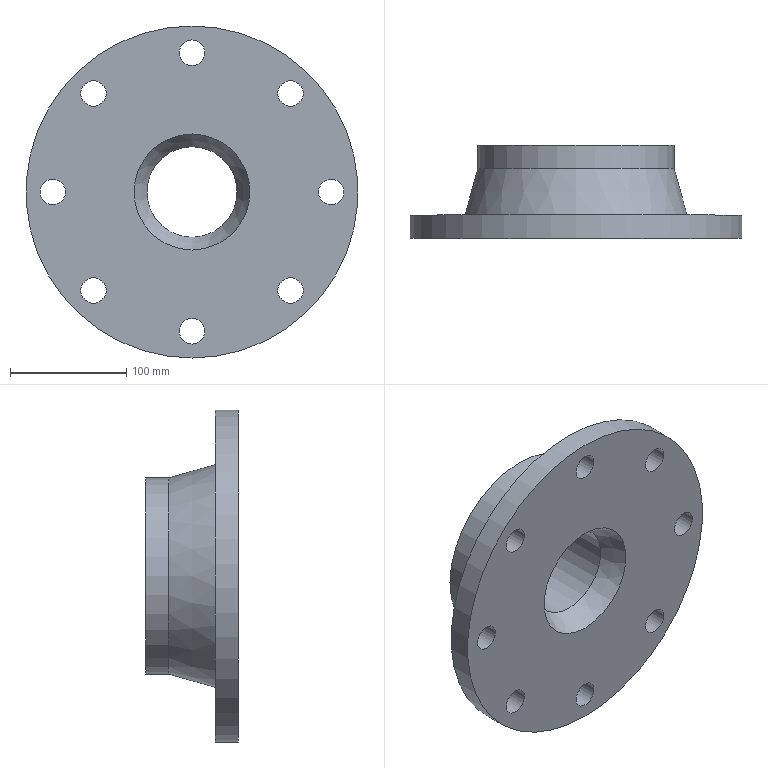Part | NX | features DATUM_CSYS 11, SKETCH 11, EXTRACT_DATUM_AXIS 8, EXTRACT_FACE 8, HOLE PACKAGE 8, SIMPLE HOLE 8, Instance Feature 7, ABSOLUTE_DATUM_PLANE 3, Resize Face 3, CPROJ 2, SWP104 2, ABSOLUTE_DATUM_AXIS 1, BLEND 1, EXTRUDE 1, Pattern Feature 1 | 2 solids | 24 faces | box 286 x 80 x 286 mm | volume 2285168 mm3 | cylinder 11 | plane 6 | cone 4 | torus 3 | commonest cylinder face diameters 22 x8 78 x1 169 x1 286 x1
STEP:
#1=CARTESIAN_POINT('',(0.,46.129,-75.847));
#2=VERTEX_POINT('',#1);
#3=CARTESIAN_POINT('',(0.,46.129,0.));
#4=DIRECTION('',(0.,-1.,0.));
#5=DIRECTION('',(0.,0.,-1.));
#6=AXIS2_PLACEMENT_3D('',#3,#4,#5);
#7=CIRCLE('',#6,75.847);
#8=EDGE_CURVE('',#2,#2,#7,.T.);
#9=ORIENTED_EDGE('',*,*,#8,.T.);
#10=EDGE_LOOP('',(#9));
#11=FACE_BOUND('',#10,.T.);
#12=CARTESIAN_POINT('',(0.,83.956,-65.03));
#13=VERTEX_POINT('',#12);
#14=CARTESIAN_POINT('',(0.,83.956,0.));
#15=DIRECTION('',(0.,-1.,0.));
#16=DIRECTION('',(0.,0.,-1.));
#17=AXIS2_PLACEMENT_3D('',#14,#15,#16);
#18=CIRCLE('',#17,65.03);
#19=EDGE_CURVE('',#13,#13,#18,.T.);
#20=ORIENTED_EDGE('',*,*,#19,.F.);
#21=EDGE_LOOP('',(#20));
#22=FACE_BOUND('',#21,.T.);
#23=CARTESIAN_POINT('',(0.,83.956,0.));
#24=DIRECTION('',(0.,-1.,0.));
#25=DIRECTION('',(0.,0.,-1.));
#26=AXIS2_PLACEMENT_3D('',#23,#24,#25);
#27=CONICAL_SURFACE('',#26,65.03,0.2785);
#28=ADVANCED_FACE('',(#11,#22),#27,.F.);
#29=CARTESIAN_POINT('',(0.,43.956,-78.73));
#30=VERTEX_POINT('',#29);
#31=CARTESIAN_POINT('',(0.,43.956,0.));
#32=DIRECTION('',(0.,-1.,0.));
#33=DIRECTION('',(0.,0.,-1.));
#34=AXIS2_PLACEMENT_3D('',#31,#32,#33);
#35=CIRCLE('',#34,78.73);
#36=EDGE_CURVE('',#30,#30,#35,.T.);
#37=ORIENTED_EDGE('',*,*,#36,.T.);
#38=EDGE_LOOP('',(#37));
#39=FACE_BOUND('',#38,.T.);
#40=ORIENTED_EDGE('',*,*,#8,.F.);
#41=EDGE_LOOP('',(#40));
#42=FACE_BOUND('',#41,.T.);
#43=CARTESIAN_POINT('',(0.,46.956,0.));
#44=DIRECTION('',(0.,-1.,0.));
#45=DIRECTION('',(0.,0.,-1.));
#46=AXIS2_PLACEMENT_3D('',#43,#44,#45);
#47=TOROIDAL_SURFACE('',#46,78.73,3.);
#48=ADVANCED_FACE('',(#39,#42),#47,.T.);
#49=CARTESIAN_POINT('',(0.,43.956,-95.938));
#50=VERTEX_POINT('',#49);
#51=CARTESIAN_POINT('',(0.,43.956,0.));
#52=DIRECTION('',(0.,-1.,0.));
#53=DIRECTION('',(0.,0.,-1.));
#54=AXIS2_PLACEMENT_3D('',#51,#52,#53);
#55=CIRCLE('',#54,95.938);
#56=EDGE_CURVE('',#50,#50,#55,.T.);
#57=ORIENTED_EDGE('',*,*,#56,.T.);
#58=EDGE_LOOP('',(#57));
#59=FACE_BOUND('',#58,.T.);
#60=ORIENTED_EDGE('',*,*,#36,.F.);
#61=EDGE_LOOP('',(#60));
#62=FACE_BOUND('',#61,.T.);
#63=CARTESIAN_POINT('',(78.73,43.956,0.));
#64=DIRECTION('',(0.,-1.,0.));
#65=DIRECTION('',(0.,0.,-1.));
#66=AXIS2_PLACEMENT_3D('',#63,#64,#65);
#67=PLANE('',#66);
#68=ADVANCED_FACE('',(#59,#62),#67,.T.);
#69=CARTESIAN_POINT('',(0.,83.956,-84.5));
#70=VERTEX_POINT('',#69);
#71=CARTESIAN_POINT('',(0.,83.956,0.));
#72=DIRECTION('',(0.,-1.,0.));
#73=DIRECTION('',(0.,0.,-1.));
#74=AXIS2_PLACEMENT_3D('',#71,#72,#73);
#75=CIRCLE('',#74,84.5);
#76=EDGE_CURVE('',#70,#70,#75,.T.);
#77=ORIENTED_EDGE('',*,*,#76,.T.);
#78=EDGE_LOOP('',(#77));
#79=FACE_BOUND('',#78,.T.);
#80=ORIENTED_EDGE('',*,*,#56,.F.);
#81=EDGE_LOOP('',(#80));
#82=FACE_BOUND('',#81,.T.);
#83=CARTESIAN_POINT('',(0.,43.956,0.));
#84=DIRECTION('',(0.,-1.,0.));
#85=DIRECTION('',(0.,0.,-1.));
#86=AXIS2_PLACEMENT_3D('',#83,#84,#85);
#87=CONICAL_SURFACE('',#86,95.938,0.2785);
#88=ADVANCED_FACE('',(#79,#82),#87,.T.);
#89=ORIENTED_EDGE('',*,*,#19,.T.);
#90=EDGE_LOOP('',(#89));
#91=FACE_BOUND('',#90,.T.);
#92=ORIENTED_EDGE('',*,*,#76,.F.);
#93=EDGE_LOOP('',(#92));
#94=FACE_BOUND('',#93,.T.);
#95=CARTESIAN_POINT('',(84.5,83.956,0.));
#96=DIRECTION('',(0.,1.,0.));
#97=DIRECTION('',(0.,0.,1.));
#98=AXIS2_PLACEMENT_3D('',#95,#96,#97);
#99=PLANE('',#98);
#100=ADVANCED_FACE('',(#91,#94),#99,.T.);
#101=CLOSED_SHELL('',(#28,#48,#68,#88,#100));
#102=MANIFOLD_SOLID_BREP('',#101);
#103=CARTESIAN_POINT('',(0.,83.55,-65.116));
#104=VERTEX_POINT('',#103);
#105=CARTESIAN_POINT('',(0.,83.55,0.));
#106=DIRECTION('',(0.,-1.,0.));
#107=DIRECTION('',(0.,0.,-1.));
#108=AXIS2_PLACEMENT_3D('',#105,#106,#107);
#109=CIRCLE('',#108,65.116);
#110=EDGE_CURVE('',#104,#104,#109,.T.);
#111=ORIENTED_EDGE('',*,*,#110,.F.);
#112=EDGE_LOOP('',(#111));
#113=FACE_BOUND('',#112,.T.);
#114=CARTESIAN_POINT('',(0.,83.956,-65.03));
#115=VERTEX_POINT('',#114);
#116=CARTESIAN_POINT('',(0.,83.956,0.));
#117=DIRECTION('',(0.,-1.,0.));
#118=DIRECTION('',(0.,0.,-1.));
#119=AXIS2_PLACEMENT_3D('',#116,#117,#118);
#120=CIRCLE('',#119,65.03);
#121=EDGE_CURVE('',#115,#115,#120,.F.);
#122=ORIENTED_EDGE('',*,*,#121,.F.);
#123=EDGE_LOOP('',(#122));
#124=FACE_BOUND('',#123,.T.);
#125=CARTESIAN_POINT('',(0.,84.377,0.));
#126=DIRECTION('',(0.,1.,0.));
#127=DIRECTION('',(0.,0.,1.));
#128=AXIS2_PLACEMENT_3D('',#125,#126,#127);
#129=TOROIDAL_SURFACE('',#128,68.,3.);
#130=ADVANCED_FACE('',(#113,#124),#129,.F.);
#131=CARTESIAN_POINT('',(-84.853,23.956,-73.853));
#132=VERTEX_POINT('',#131);
#133=CARTESIAN_POINT('',(-84.853,23.956,-84.853));
#134=DIRECTION('',(0.,1.,0.));
#135=DIRECTION('',(0.,0.,1.));
#136=AXIS2_PLACEMENT_3D('',#133,#134,#135);
#137=CIRCLE('',#136,11.);
#138=EDGE_CURVE('',#132,#132,#137,.T.);
#139=ORIENTED_EDGE('',*,*,#138,.T.);
#140=EDGE_LOOP('',(#139));
#141=FACE_BOUND('',#140,.T.);
#142=CARTESIAN_POINT('',(0.,23.956,-109.));
#143=VERTEX_POINT('',#142);
#144=CARTESIAN_POINT('',(0.,23.956,-120.));
#145=DIRECTION('',(0.,1.,0.));
#146=DIRECTION('',(0.,0.,1.));
#147=AXIS2_PLACEMENT_3D('',#144,#145,#146);
#148=CIRCLE('',#147,11.);
#149=EDGE_CURVE('',#143,#143,#148,.T.);
#150=ORIENTED_EDGE('',*,*,#149,.T.);
#151=EDGE_LOOP('',(#150));
#152=FACE_BOUND('',#151,.T.);
#153=CARTESIAN_POINT('',(84.853,23.956,-73.853));
#154=VERTEX_POINT('',#153);
#155=CARTESIAN_POINT('',(84.853,23.956,-84.853));
#156=DIRECTION('',(0.,1.,0.));
#157=DIRECTION('',(0.,0.,1.));
#158=AXIS2_PLACEMENT_3D('',#155,#156,#157);
#159=CIRCLE('',#158,11.);
#160=EDGE_CURVE('',#154,#154,#159,.T.);
#161=ORIENTED_EDGE('',*,*,#160,.T.);
#162=EDGE_LOOP('',(#161));
#163=FACE_BOUND('',#162,.T.);
#164=CARTESIAN_POINT('',(120.,23.956,11.));
#165=VERTEX_POINT('',#164);
#166=CARTESIAN_POINT('',(120.,23.956,0.));
#167=DIRECTION('',(0.,1.,0.));
#168=DIRECTION('',(0.,0.,1.));
#169=AXIS2_PLACEMENT_3D('',#166,#167,#168);
#170=CIRCLE('',#169,11.);
#171=EDGE_CURVE('',#165,#165,#170,.T.);
#172=ORIENTED_EDGE('',*,*,#171,.T.);
#173=EDGE_LOOP('',(#172));
#174=FACE_BOUND('',#173,.T.);
#175=CARTESIAN_POINT('',(84.853,23.956,95.853));
#176=VERTEX_POINT('',#175);
#177=CARTESIAN_POINT('',(84.853,23.956,84.853));
#178=DIRECTION('',(0.,1.,0.));
#179=DIRECTION('',(0.,0.,1.));
#180=AXIS2_PLACEMENT_3D('',#177,#178,#179);
#181=CIRCLE('',#180,11.);
#182=EDGE_CURVE('',#176,#176,#181,.T.);
#183=ORIENTED_EDGE('',*,*,#182,.T.);
#184=EDGE_LOOP('',(#183));
#185=FACE_BOUND('',#184,.T.);
#186=CARTESIAN_POINT('',(0.,23.956,131.));
#187=VERTEX_POINT('',#186);
#188=CARTESIAN_POINT('',(0.,23.956,120.));
#189=DIRECTION('',(0.,1.,0.));
#190=DIRECTION('',(0.,0.,1.));
#191=AXIS2_PLACEMENT_3D('',#188,#189,#190);
#192=CIRCLE('',#191,11.);
#193=EDGE_CURVE('',#187,#187,#192,.T.);
#194=ORIENTED_EDGE('',*,*,#193,.T.);
#195=EDGE_LOOP('',(#194));
#196=FACE_BOUND('',#195,.T.);
#197=CARTESIAN_POINT('',(-84.853,23.956,95.853));
#198=VERTEX_POINT('',#197);
#199=CARTESIAN_POINT('',(-84.853,23.956,84.853));
#200=DIRECTION('',(0.,1.,0.));
#201=DIRECTION('',(0.,0.,1.));
#202=AXIS2_PLACEMENT_3D('',#199,#200,#201);
#203=CIRCLE('',#202,11.);
#204=EDGE_CURVE('',#198,#198,#203,.T.);
#205=ORIENTED_EDGE('',*,*,#204,.T.);
#206=EDGE_LOOP('',(#205));
#207=FACE_BOUND('',#206,.T.);
#208=CARTESIAN_POINT('',(-120.,23.956,11.));
#209=VERTEX_POINT('',#208);
#210=CARTESIAN_POINT('',(-120.,23.956,0.));
#211=DIRECTION('',(0.,1.,0.));
#212=DIRECTION('',(0.,0.,1.));
#213=AXIS2_PLACEMENT_3D('',#210,#211,#212);
#214=CIRCLE('',#213,11.);
#215=EDGE_CURVE('',#209,#209,#214,.T.);
#216=ORIENTED_EDGE('',*,*,#215,.T.);
#217=EDGE_LOOP('',(#216));
#218=FACE_BOUND('',#217,.T.);
#219=CARTESIAN_POINT('',(0.,23.956,-50.));
#220=VERTEX_POINT('',#219);
#221=CARTESIAN_POINT('',(0.,23.956,0.));
#222=DIRECTION('',(0.,-1.,0.));
#223=DIRECTION('',(0.,0.,-1.));
#224=AXIS2_PLACEMENT_3D('',#221,#222,#223);
#225=CIRCLE('',#224,50.);
#226=EDGE_CURVE('',#220,#220,#225,.T.);
#227=ORIENTED_EDGE('',*,*,#226,.F.);
#228=EDGE_LOOP('',(#227));
#229=FACE_BOUND('',#228,.T.);
#230=CARTESIAN_POINT('',(0.,23.956,143.));
#231=VERTEX_POINT('',#230);
#232=CARTESIAN_POINT('',(0.,23.956,0.));
#233=DIRECTION('',(0.,1.,0.));
#234=DIRECTION('',(0.,0.,1.));
#235=AXIS2_PLACEMENT_3D('',#232,#233,#234);
#236=CIRCLE('',#235,143.);
#237=EDGE_CURVE('',#231,#231,#236,.F.);
#238=ORIENTED_EDGE('',*,*,#237,.T.);
#239=EDGE_LOOP('',(#238));
#240=FACE_BOUND('',#239,.T.);
#241=CARTESIAN_POINT('',(110.,23.956,0.));
#242=DIRECTION('',(0.,1.,0.));
#243=DIRECTION('',(0.,0.,1.));
#244=AXIS2_PLACEMENT_3D('',#241,#242,#243);
#245=PLANE('',#244);
#246=ADVANCED_FACE('',(#141,#152,#163,#174,#185,#196,#207,#218,#229,#240),#245,.F.);
#247=CARTESIAN_POINT('',(0.,43.756,-39.));
#248=VERTEX_POINT('',#247);
#249=CARTESIAN_POINT('',(0.,43.756,0.));
#250=DIRECTION('',(0.,-1.,0.));
#251=DIRECTION('',(0.,0.,-1.));
#252=AXIS2_PLACEMENT_3D('',#249,#250,#251);
#253=CIRCLE('',#252,39.);
#254=EDGE_CURVE('',#248,#248,#253,.T.);
#255=ORIENTED_EDGE('',*,*,#254,.F.);
#256=EDGE_LOOP('',(#255));
#257=FACE_BOUND('',#256,.T.);
#258=ORIENTED_EDGE('',*,*,#226,.T.);
#259=EDGE_LOOP('',(#258));
#260=FACE_BOUND('',#259,.T.);
#261=CARTESIAN_POINT('',(0.,23.956,0.));
#262=DIRECTION('',(0.,-1.,0.));
#263=DIRECTION('',(0.,0.,-1.));
#264=AXIS2_PLACEMENT_3D('',#261,#262,#263);
#265=CONICAL_SURFACE('',#264,50.,0.5071);
#266=ADVANCED_FACE('',(#257,#260),#265,.F.);
#267=CARTESIAN_POINT('',(0.,103.956,-39.));
#268=VERTEX_POINT('',#267);
#269=CARTESIAN_POINT('',(0.,103.956,0.));
#270=DIRECTION('',(0.,-1.,0.));
#271=DIRECTION('',(0.,0.,-1.));
#272=AXIS2_PLACEMENT_3D('',#269,#270,#271);
#273=CIRCLE('',#272,39.);
#274=EDGE_CURVE('',#268,#268,#273,.T.);
#275=ORIENTED_EDGE('',*,*,#274,.F.);
#276=EDGE_LOOP('',(#275));
#277=FACE_BOUND('',#276,.T.);
#278=ORIENTED_EDGE('',*,*,#254,.T.);
#279=EDGE_LOOP('',(#278));
#280=FACE_BOUND('',#279,.T.);
#281=CARTESIAN_POINT('',(0.,0.,0.));
#282=DIRECTION('',(0.,-1.,0.));
#283=DIRECTION('',(0.,0.,-1.));
#284=AXIS2_PLACEMENT_3D('',#281,#282,#283);
#285=CYLINDRICAL_SURFACE('',#284,39.);
#286=ADVANCED_FACE('',(#277,#280),#285,.F.);
#287=ORIENTED_EDGE('',*,*,#274,.T.);
#288=EDGE_LOOP('',(#287));
#289=FACE_BOUND('',#288,.T.);
#290=CARTESIAN_POINT('',(0.,103.956,84.5));
#291=VERTEX_POINT('',#290);
#292=CARTESIAN_POINT('',(0.,103.956,0.));
#293=DIRECTION('',(0.,1.,0.));
#294=DIRECTION('',(0.,0.,1.));
#295=AXIS2_PLACEMENT_3D('',#292,#293,#294);
#296=CIRCLE('',#295,84.5);
#297=EDGE_CURVE('',#291,#291,#296,.T.);
#298=ORIENTED_EDGE('',*,*,#297,.T.);
#299=EDGE_LOOP('',(#298));
#300=FACE_BOUND('',#299,.T.);
#301=CARTESIAN_POINT('',(20.,103.956,0.));
#302=DIRECTION('',(0.,-1.,0.));
#303=DIRECTION('',(0.,0.,-1.));
#304=AXIS2_PLACEMENT_3D('',#301,#302,#303);
#305=PLANE('',#304);
#306=ADVANCED_FACE('',(#289,#300),#305,.F.);
#307=CARTESIAN_POINT('',(0.,46.129,-75.847));
#308=VERTEX_POINT('',#307);
#309=CARTESIAN_POINT('',(0.,46.129,0.));
#310=DIRECTION('',(0.,-1.,0.));
#311=DIRECTION('',(0.,0.,-1.));
#312=AXIS2_PLACEMENT_3D('',#309,#310,#311);
#313=CIRCLE('',#312,75.847);
#314=EDGE_CURVE('',#308,#308,#313,.F.);
#315=ORIENTED_EDGE('',*,*,#314,.T.);
#316=EDGE_LOOP('',(#315));
#317=FACE_BOUND('',#316,.T.);
#318=ORIENTED_EDGE('',*,*,#110,.T.);
#319=EDGE_LOOP('',(#318));
#320=FACE_BOUND('',#319,.T.);
#321=CARTESIAN_POINT('',(0.,83.956,0.));
#322=DIRECTION('',(0.,-1.,0.));
#323=DIRECTION('',(0.,0.,-1.));
#324=AXIS2_PLACEMENT_3D('',#321,#322,#323);
#325=CONICAL_SURFACE('',#324,65.,0.2793);
#326=ADVANCED_FACE('',(#317,#320),#325,.T.);
#327=CARTESIAN_POINT('',(-84.853,43.956,-95.853));
#328=VERTEX_POINT('',#327);
#329=CARTESIAN_POINT('',(-84.853,43.956,-84.853));
#330=DIRECTION('',(0.,-1.,0.));
#331=DIRECTION('',(0.,0.,-1.));
#332=AXIS2_PLACEMENT_3D('',#329,#330,#331);
#333=CIRCLE('',#332,11.);
#334=EDGE_CURVE('',#328,#328,#333,.T.);
#335=ORIENTED_EDGE('',*,*,#334,.T.);
#336=EDGE_LOOP('',(#335));
#337=FACE_BOUND('',#336,.T.);
#338=CARTESIAN_POINT('',(0.,43.956,-131.));
#339=VERTEX_POINT('',#338);
#340=CARTESIAN_POINT('',(0.,43.956,-120.));
#341=DIRECTION('',(0.,-1.,0.));
#342=DIRECTION('',(0.,0.,-1.));
#343=AXIS2_PLACEMENT_3D('',#340,#341,#342);
#344=CIRCLE('',#343,11.);
#345=EDGE_CURVE('',#339,#339,#344,.T.);
#346=ORIENTED_EDGE('',*,*,#345,.T.);
#347=EDGE_LOOP('',(#346));
#348=FACE_BOUND('',#347,.T.);
#349=CARTESIAN_POINT('',(84.853,43.956,-95.853));
#350=VERTEX_POINT('',#349);
#351=CARTESIAN_POINT('',(84.853,43.956,-84.853));
#352=DIRECTION('',(0.,-1.,0.));
#353=DIRECTION('',(0.,0.,-1.));
#354=AXIS2_PLACEMENT_3D('',#351,#352,#353);
#355=CIRCLE('',#354,11.);
#356=EDGE_CURVE('',#350,#350,#355,.T.);
#357=ORIENTED_EDGE('',*,*,#356,.T.);
#358=EDGE_LOOP('',(#357));
#359=FACE_BOUND('',#358,.T.);
#360=CARTESIAN_POINT('',(120.,43.956,-11.));
#361=VERTEX_POINT('',#360);
#362=CARTESIAN_POINT('',(120.,43.956,0.));
#363=DIRECTION('',(0.,-1.,0.));
#364=DIRECTION('',(0.,0.,-1.));
#365=AXIS2_PLACEMENT_3D('',#362,#363,#364);
#366=CIRCLE('',#365,11.);
#367=EDGE_CURVE('',#361,#361,#366,.T.);
#368=ORIENTED_EDGE('',*,*,#367,.T.);
#369=EDGE_LOOP('',(#368));
#370=FACE_BOUND('',#369,.T.);
#371=CARTESIAN_POINT('',(84.853,43.956,73.853));
#372=VERTEX_POINT('',#371);
#373=CARTESIAN_POINT('',(84.853,43.956,84.853));
#374=DIRECTION('',(0.,-1.,0.));
#375=DIRECTION('',(0.,0.,-1.));
#376=AXIS2_PLACEMENT_3D('',#373,#374,#375);
#377=CIRCLE('',#376,11.);
#378=EDGE_CURVE('',#372,#372,#377,.T.);
#379=ORIENTED_EDGE('',*,*,#378,.T.);
#380=EDGE_LOOP('',(#379));
#381=FACE_BOUND('',#380,.T.);
#382=CARTESIAN_POINT('',(0.,43.956,109.));
#383=VERTEX_POINT('',#382);
#384=CARTESIAN_POINT('',(0.,43.956,120.));
#385=DIRECTION('',(0.,-1.,0.));
#386=DIRECTION('',(0.,0.,-1.));
#387=AXIS2_PLACEMENT_3D('',#384,#385,#386);
#388=CIRCLE('',#387,11.);
#389=EDGE_CURVE('',#383,#383,#388,.T.);
#390=ORIENTED_EDGE('',*,*,#389,.T.);
#391=EDGE_LOOP('',(#390));
#392=FACE_BOUND('',#391,.T.);
#393=CARTESIAN_POINT('',(-84.853,43.956,73.853));
#394=VERTEX_POINT('',#393);
#395=CARTESIAN_POINT('',(-84.853,43.956,84.853));
#396=DIRECTION('',(0.,-1.,0.));
#397=DIRECTION('',(0.,0.,-1.));
#398=AXIS2_PLACEMENT_3D('',#395,#396,#397);
#399=CIRCLE('',#398,11.);
#400=EDGE_CURVE('',#394,#394,#399,.T.);
#401=ORIENTED_EDGE('',*,*,#400,.T.);
#402=EDGE_LOOP('',(#401));
#403=FACE_BOUND('',#402,.T.);
#404=CARTESIAN_POINT('',(-120.,43.956,-11.));
#405=VERTEX_POINT('',#404);
#406=CARTESIAN_POINT('',(-120.,43.956,0.));
#407=DIRECTION('',(0.,-1.,0.));
#408=DIRECTION('',(0.,0.,-1.));
#409=AXIS2_PLACEMENT_3D('',#406,#407,#408);
#410=CIRCLE('',#409,11.);
#411=EDGE_CURVE('',#405,#405,#410,.T.);
#412=ORIENTED_EDGE('',*,*,#411,.T.);
#413=EDGE_LOOP('',(#412));
#414=FACE_BOUND('',#413,.T.);
#415=CARTESIAN_POINT('',(0.,43.956,-78.73));
#416=VERTEX_POINT('',#415);
#417=CARTESIAN_POINT('',(0.,43.956,0.));
#418=DIRECTION('',(0.,-1.,0.));
#419=DIRECTION('',(0.,0.,-1.));
#420=AXIS2_PLACEMENT_3D('',#417,#418,#419);
#421=CIRCLE('',#420,78.73);
#422=EDGE_CURVE('',#416,#416,#421,.T.);
#423=ORIENTED_EDGE('',*,*,#422,.T.);
#424=EDGE_LOOP('',(#423));
#425=FACE_BOUND('',#424,.T.);
#426=CARTESIAN_POINT('',(0.,43.956,-143.));
#427=VERTEX_POINT('',#426);
#428=CARTESIAN_POINT('',(0.,43.956,0.));
#429=DIRECTION('',(0.,-1.,0.));
#430=DIRECTION('',(0.,0.,-1.));
#431=AXIS2_PLACEMENT_3D('',#428,#429,#430);
#432=CIRCLE('',#431,143.);
#433=EDGE_CURVE('',#427,#427,#432,.T.);
#434=ORIENTED_EDGE('',*,*,#433,.F.);
#435=EDGE_LOOP('',(#434));
#436=FACE_BOUND('',#435,.T.);
#437=CARTESIAN_POINT('',(75.,43.956,0.));
#438=DIRECTION('',(0.,-1.,0.));
#439=DIRECTION('',(0.,0.,-1.));
#440=AXIS2_PLACEMENT_3D('',#437,#438,#439);
#441=PLANE('',#440);
#442=ADVANCED_FACE('',(#337,#348,#359,#370,#381,#392,#403,#414,#425,#436),#441,.F.);
#443=ORIENTED_EDGE('',*,*,#237,.F.);
#444=EDGE_LOOP('',(#443));
#445=FACE_BOUND('',#444,.T.);
#446=ORIENTED_EDGE('',*,*,#433,.T.);
#447=EDGE_LOOP('',(#446));
#448=FACE_BOUND('',#447,.T.);
#449=CARTESIAN_POINT('',(0.,0.,0.));
#450=DIRECTION('',(0.,-1.,0.));
#451=DIRECTION('',(0.,0.,-1.));
#452=AXIS2_PLACEMENT_3D('',#449,#450,#451);
#453=CYLINDRICAL_SURFACE('',#452,143.);
#454=ADVANCED_FACE('',(#445,#448),#453,.T.);
#455=ORIENTED_EDGE('',*,*,#314,.F.);
#456=EDGE_LOOP('',(#455));
#457=FACE_BOUND('',#456,.T.);
#458=ORIENTED_EDGE('',*,*,#422,.F.);
#459=EDGE_LOOP('',(#458));
#460=FACE_BOUND('',#459,.T.);
#461=CARTESIAN_POINT('',(0.,46.956,0.));
#462=DIRECTION('',(0.,-1.,0.));
#463=DIRECTION('',(0.,0.,-1.));
#464=AXIS2_PLACEMENT_3D('',#461,#462,#463);
#465=TOROIDAL_SURFACE('',#464,78.73,3.);
#466=ADVANCED_FACE('',(#457,#460),#465,.F.);
#467=ORIENTED_EDGE('',*,*,#411,.F.);
#468=EDGE_LOOP('',(#467));
#469=FACE_BOUND('',#468,.T.);
#470=ORIENTED_EDGE('',*,*,#215,.F.);
#471=EDGE_LOOP('',(#470));
#472=FACE_BOUND('',#471,.T.);
#473=CARTESIAN_POINT('',(-120.,43.956,0.));
#474=DIRECTION('',(0.,-1.,0.));
#475=DIRECTION('',(0.,0.,-1.));
#476=AXIS2_PLACEMENT_3D('',#473,#474,#475);
#477=CYLINDRICAL_SURFACE('',#476,11.);
#478=ADVANCED_FACE('',(#469,#472),#477,.F.);
#479=ORIENTED_EDGE('',*,*,#400,.F.);
#480=EDGE_LOOP('',(#479));
#481=FACE_BOUND('',#480,.T.);
#482=ORIENTED_EDGE('',*,*,#204,.F.);
#483=EDGE_LOOP('',(#482));
#484=FACE_BOUND('',#483,.T.);
#485=CARTESIAN_POINT('',(-84.853,43.956,84.853));
#486=DIRECTION('',(0.,-1.,0.));
#487=DIRECTION('',(0.,0.,-1.));
#488=AXIS2_PLACEMENT_3D('',#485,#486,#487);
#489=CYLINDRICAL_SURFACE('',#488,11.);
#490=ADVANCED_FACE('',(#481,#484),#489,.F.);
#491=ORIENTED_EDGE('',*,*,#389,.F.);
#492=EDGE_LOOP('',(#491));
#493=FACE_BOUND('',#492,.T.);
#494=ORIENTED_EDGE('',*,*,#193,.F.);
#495=EDGE_LOOP('',(#494));
#496=FACE_BOUND('',#495,.T.);
#497=CARTESIAN_POINT('',(0.,43.956,120.));
#498=DIRECTION('',(0.,-1.,0.));
#499=DIRECTION('',(0.,0.,-1.));
#500=AXIS2_PLACEMENT_3D('',#497,#498,#499);
#501=CYLINDRICAL_SURFACE('',#500,11.);
#502=ADVANCED_FACE('',(#493,#496),#501,.F.);
#503=ORIENTED_EDGE('',*,*,#378,.F.);
#504=EDGE_LOOP('',(#503));
#505=FACE_BOUND('',#504,.T.);
#506=ORIENTED_EDGE('',*,*,#182,.F.);
#507=EDGE_LOOP('',(#506));
#508=FACE_BOUND('',#507,.T.);
#509=CARTESIAN_POINT('',(84.853,43.956,84.853));
#510=DIRECTION('',(0.,-1.,0.));
#511=DIRECTION('',(0.,0.,-1.));
#512=AXIS2_PLACEMENT_3D('',#509,#510,#511);
#513=CYLINDRICAL_SURFACE('',#512,11.);
#514=ADVANCED_FACE('',(#505,#508),#513,.F.);
#515=ORIENTED_EDGE('',*,*,#367,.F.);
#516=EDGE_LOOP('',(#515));
#517=FACE_BOUND('',#516,.T.);
#518=ORIENTED_EDGE('',*,*,#171,.F.);
#519=EDGE_LOOP('',(#518));
#520=FACE_BOUND('',#519,.T.);
#521=CARTESIAN_POINT('',(120.,43.956,0.));
#522=DIRECTION('',(0.,-1.,0.));
#523=DIRECTION('',(0.,0.,-1.));
#524=AXIS2_PLACEMENT_3D('',#521,#522,#523);
#525=CYLINDRICAL_SURFACE('',#524,11.);
#526=ADVANCED_FACE('',(#517,#520),#525,.F.);
#527=ORIENTED_EDGE('',*,*,#356,.F.);
#528=EDGE_LOOP('',(#527));
#529=FACE_BOUND('',#528,.T.);
#530=ORIENTED_EDGE('',*,*,#160,.F.);
#531=EDGE_LOOP('',(#530));
#532=FACE_BOUND('',#531,.T.);
#533=CARTESIAN_POINT('',(84.853,43.956,-84.853));
#534=DIRECTION('',(0.,-1.,0.));
#535=DIRECTION('',(0.,0.,-1.));
#536=AXIS2_PLACEMENT_3D('',#533,#534,#535);
#537=CYLINDRICAL_SURFACE('',#536,11.);
#538=ADVANCED_FACE('',(#529,#532),#537,.F.);
#539=ORIENTED_EDGE('',*,*,#345,.F.);
#540=EDGE_LOOP('',(#539));
#541=FACE_BOUND('',#540,.T.);
#542=ORIENTED_EDGE('',*,*,#149,.F.);
#543=EDGE_LOOP('',(#542));
#544=FACE_BOUND('',#543,.T.);
#545=CARTESIAN_POINT('',(0.,43.956,-120.));
#546=DIRECTION('',(0.,-1.,0.));
#547=DIRECTION('',(0.,0.,-1.));
#548=AXIS2_PLACEMENT_3D('',#545,#546,#547);
#549=CYLINDRICAL_SURFACE('',#548,11.);
#550=ADVANCED_FACE('',(#541,#544),#549,.F.);
#551=ORIENTED_EDGE('',*,*,#334,.F.);
#552=EDGE_LOOP('',(#551));
#553=FACE_BOUND('',#552,.T.);
#554=ORIENTED_EDGE('',*,*,#138,.F.);
#555=EDGE_LOOP('',(#554));
#556=FACE_BOUND('',#555,.T.);
#557=CARTESIAN_POINT('',(-84.853,43.956,-84.853));
#558=DIRECTION('',(0.,-1.,0.));
#559=DIRECTION('',(0.,0.,-1.));
#560=AXIS2_PLACEMENT_3D('',#557,#558,#559);
#561=CYLINDRICAL_SURFACE('',#560,11.);
#562=ADVANCED_FACE('',(#553,#556),#561,.F.);
#563=CARTESIAN_POINT('',(0.,83.956,84.5));
#564=VERTEX_POINT('',#563);
#565=CARTESIAN_POINT('',(0.,83.956,0.));
#566=DIRECTION('',(0.,1.,0.));
#567=DIRECTION('',(0.,0.,1.));
#568=AXIS2_PLACEMENT_3D('',#565,#566,#567);
#569=CIRCLE('',#568,84.5);
#570=EDGE_CURVE('',#564,#564,#569,.T.);
#571=ORIENTED_EDGE('',*,*,#570,.T.);
#572=EDGE_LOOP('',(#571));
#573=FACE_BOUND('',#572,.T.);
#574=ORIENTED_EDGE('',*,*,#297,.F.);
#575=EDGE_LOOP('',(#574));
#576=FACE_BOUND('',#575,.T.);
#577=CARTESIAN_POINT('',(0.,83.956,0.));
#578=DIRECTION('',(0.,1.,0.));
#579=DIRECTION('',(0.,0.,1.));
#580=AXIS2_PLACEMENT_3D('',#577,#578,#579);
#581=CYLINDRICAL_SURFACE('',#580,84.5);
#582=ADVANCED_FACE('',(#573,#576),#581,.T.);
#583=ORIENTED_EDGE('',*,*,#121,.T.);
#584=EDGE_LOOP('',(#583));
#585=FACE_BOUND('',#584,.T.);
#586=ORIENTED_EDGE('',*,*,#570,.F.);
#587=EDGE_LOOP('',(#586));
#588=FACE_BOUND('',#587,.T.);
#589=CARTESIAN_POINT('',(0.,83.956,0.));
#590=DIRECTION('',(0.,1.,0.));
#591=DIRECTION('',(0.,0.,1.));
#592=AXIS2_PLACEMENT_3D('',#589,#590,#591);
#593=PLANE('',#592);
#594=ADVANCED_FACE('',(#585,#588),#593,.F.);
#595=CLOSED_SHELL('',(#130,#246,#266,#286,#306,#326,#442,#454,#466,#478,#490,#502,#514,#526,#538,#550,#562,#582,#594));
#596=MANIFOLD_SOLID_BREP('',#595);
#597=(LENGTH_UNIT()NAMED_UNIT(*)SI_UNIT(.MILLI.,.METRE.));
#598=UNCERTAINTY_MEASURE_WITH_UNIT(LENGTH_MEASURE(0.00001),#597,'','');
#599=(NAMED_UNIT(*)PLANE_ANGLE_UNIT()SI_UNIT($,.RADIAN.));
#600=(NAMED_UNIT(*)SI_UNIT($,.STERADIAN.)SOLID_ANGLE_UNIT());
#601=(GEOMETRIC_REPRESENTATION_CONTEXT(3)GLOBAL_UNCERTAINTY_ASSIGNED_CONTEXT((#598))GLOBAL_UNIT_ASSIGNED_CONTEXT((#597,#599,#600))REPRESENTATION_CONTEXT('',''));
#602=ADVANCED_BREP_SHAPE_REPRESENTATION('',(#102,#596),#601);